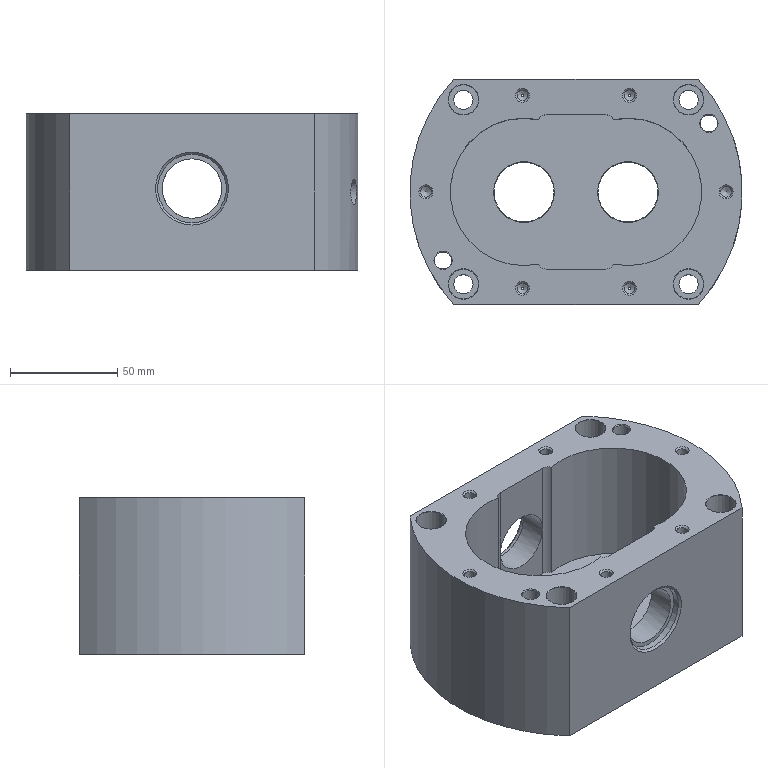NC program | NX | posted with a generic post | part box 155 x 105 x 73.2 mm
Lines 1 to 85 of 150882:
N10 G17 G21 G94 G90
(DRILLING , TOOL : ZXZ)
N12 T01 M6
N14 G54
N16 G17 G0 G90 X-52.5 Y43. B0. C0. S5000 M3
N18 G43 Z30. H1
N20 G94 G81 G98 Z-1. F250. R3.
N22 X-62. Y32.
N24 X-42.918 Y18.668
N26 X-24.25 Y0.
N28 X-42.918 Y-18.668
N30 X-52.5 Y-43.
N32 X-5.582 Y-18.668
N34 X5.582
N36 X-5.582 Y18.668
N38 X5.582
N40 X52.5 Y43.
N42 X42.918 Y18.668
N44 X24.25 Y0.
N46 X42.918 Y-18.668
N48 X62. Y-32.
N50 X52.5 Y-43.
N52 G80
N54 G0 X52.5 Y-43. Z30.
N56 M5
(DRILLING_COPY , TOOL : 9.0ZT)
N58 T09 M6
N60 G54
N62 G17 G0 G90 X-52.5 Y43. B0. C0. S2000 M3
N64 G43 Z30. H9
N66 G94 G83 G98 Z-70.104 F150. Q2. R3.
N68 Y-43.
N70 X52.5
N72 Y43.
N74 G80
N76 G0 X52.5 Y43. Z30.
N78 M5
(DRILLING_COPY_COPY , TOOL : 7.8ZT)
N80 T19 M6
N82 G54
N84 G17 G0 G90 X-62. Y32. B0. C0. S2000 M3
N86 G43 Z30. H19
N88 G94 G83 G98 Z-77.043 F150. Q2. R3.
N90 X62. Y-32.
N92 G80
N94 G0 X62. Y-32. Z30.
N96 M5
(DRILLING_COPY_COPY_COPY , TOOL : 8.0JD)
N98 T17 M6
N100 G54
N102 G17 G0 G90 X-62. Y32. B0. C0. S800 M3
N104 G43 Z30. H17
N106 G94 G85 G98 Z-73.7 F40. R3.
N108 X62. Y-32.
N110 G80
N112 G0 X62. Y-32. Z30.
N114 M5
(DRILLING_COPY_COPY_1 , TOOL : 5.0ZT)
N116 T15 M6
N118 G54
N120 G17 G0 G90 X42.918 Y18.668 B0. C0. S2000 M3
N122 G43 Z30. H15
N124 G94 G83 G98 Z-10.002 F150. Q2. R3.
N126 Y-18.668
N128 X5.582
N130 X-5.582
N132 X-42.918
N134 Y18.668
N136 X-5.582
N138 X5.582
N140 G80
N142 G0 X5.582 Y18.668 Z30.
N144 M5